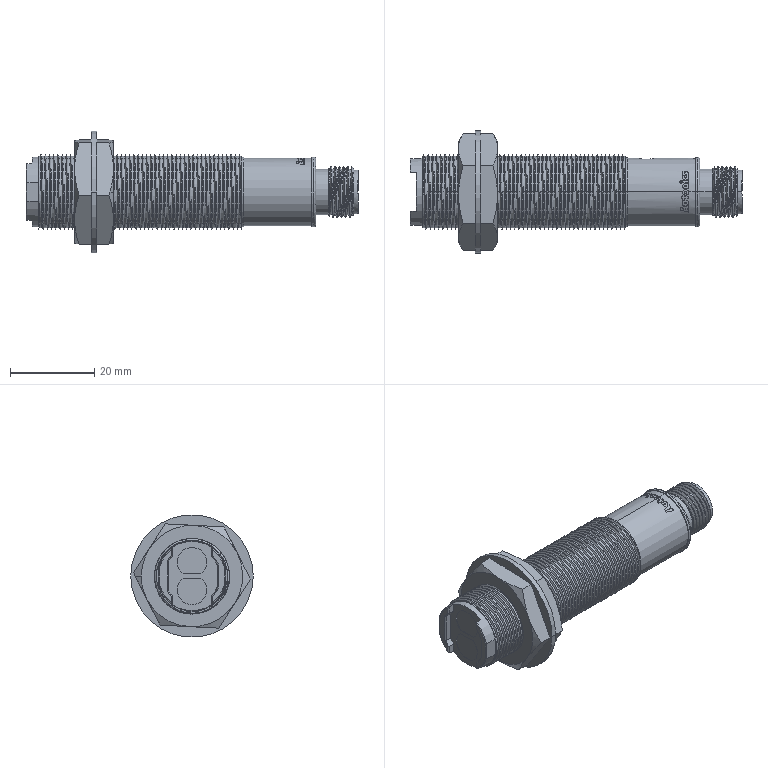Part | SolidWorks | features BaseBody 4 | 4 solids | 529 faces | box 78.6 x 29 x 29 mm | volume 17778 mm3 | cylinder 234 | plane 198 | spline 60 | cone 37 | commonest cylinder face diameters 16.9 x98 16.92 x20 24 x13 19 x12 12 x11 15.98 x10